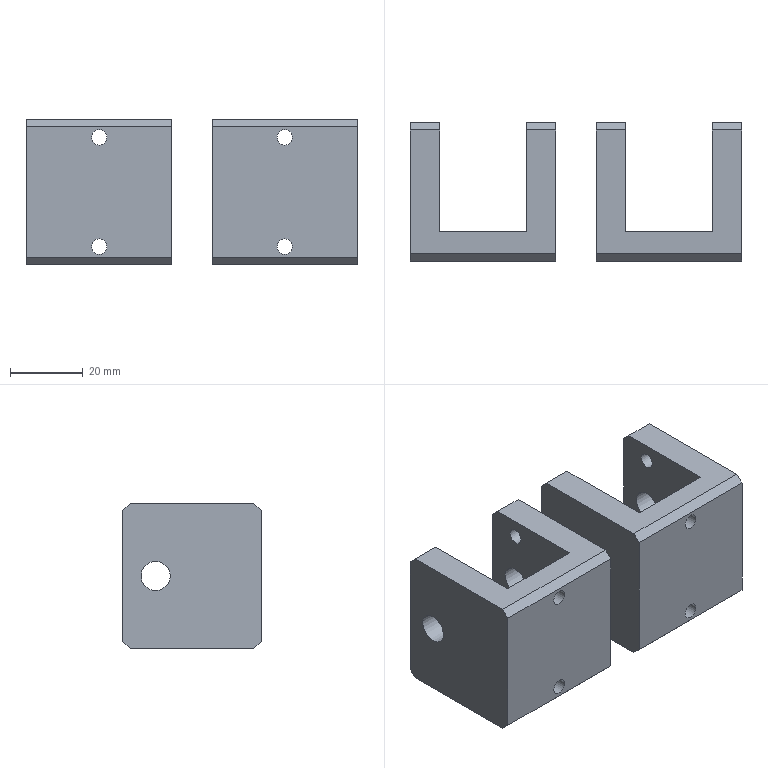NC program | NX | posted by the shop | part box 91 x 38 x 40 mm
Whole program:
%
O0001
(Machine time: 2.39 MIN)
(===Total Tool:3===)
(T1=D80R0.8 face mill D=80.  R=0.8  D-  H01 Z=0.    )
(T9=D10     D=10.  R=0.   D-  H09 Z=-2.   )
(T2=D6 chamfer mill   D=6.   R=0.   D-  H02 Z=-2.7  )
G80 G90 G17 G49 G40
G91 G28 Z0
M01
N1 T01 M06
(D80R0.8 face mill  D=80. R=0.8 H=01 ce=0.10 di=0.10)
G00 G90 G54 X97.597 Y-20. M03 S2800
G43 H01 Z20.
M08
Z3.525
G01 Z1.525 F3000.
X85.597
X-85.597
X-97.597
Z3.525
G00 X97.597
Z3.05
G01 Z1.05
X85.597
X-85.597
X-97.597
Z3.05
G00 X97.597
Z2.575
G01 Z.575
X85.597
X-85.597
X-97.597
Z2.575
G00 X97.597
Z2.1
G01 Z.1
X85.597
X-85.597
X-97.597
Z2.1
G00 Z20.
G91 G28 Z0.0
M05
M09
G91 G28 Z0.0
M01
N2 T01 M06
(D80R0.8 face mill-J  D=80. R=0.8 H=01 ce=0.00 di=0.00)
G00 G90 G54 X97.499 Y-20. M03 S4000
G43 H01 Z20.
M08
Z2.
G01 Z0.0 F1000.
X85.499
X-85.499
X-97.499
Z2.
G00 Z20.
G91 G28 Z0.0
M05
M09
G91 G28 Z0.0
M01
N3 T09 M06
(D10  D=10. R=0. H=09 ce=0.10 di=0.00)
G00 G90 G54 X0.0 Y7.219 M03 S7000
G43 H09 Z11.8
M08
Z.359
G01 Z-.141 F4000.
X-.57 Y3.093
X4.428 Y3.239
X4.513 Y3.241
X46.485
X46.572 Y3.239
Y3.312 Z-.212
Y3.38 Z-.283
X46.485 Y3.383
X4.513
X4.428 Y3.38
Y3.454 Z-.354
Y3.522 Z-.424
X4.513 Y3.524
X46.485
X46.572 Y3.522
X46.573 Y3.595 Z-.495
Y3.663 Z-.566
X46.485 Y3.666
X4.513
X4.428 Y3.663
X4.427 Y3.736 Z-.636
Y3.805 Z-.707
X4.513 Y3.807
X46.485
X46.573 Y3.805
Y3.878 Z-.778
Y3.946 Z-.849
X46.485 Y3.949
X4.513
X4.427 Y3.946
Y4.019 Z-.919
Y4.087 Z-.99
X4.513 Y4.09
X46.485
X46.573 Y4.087
Y4.161 Z-1.061
Y4.229 Z-1.131
X46.485 Y4.231
X4.513
X4.427 Y4.229
Y4.302 Z-1.202
Y4.37 Z-1.273
X4.513 Y4.373
X46.485
X46.573 Y4.37
Y4.444 Z-1.344
Y4.512 Z-1.414
X46.485 Y4.514
X4.513
X4.427 Y4.512
Y4.585 Z-1.485
X4.428 Y4.653 Z-1.556
X4.513 Y4.656
X46.485
X46.572 Y4.653
Y4.711 Z-1.611
Y4.764 Z-1.667
X46.485 Y4.767
X4.513
X4.428 Y4.764
Y4.822 Z-1.722
Y4.875 Z-1.778
X4.513 Y4.878
X46.485
X46.572 Y4.875
Y4.933 Z-1.833
Y4.986 Z-1.889
X46.485 Y4.989
X4.513
X4.428 Y4.986
Y5.044 Z-1.944
Y5.098 Z-2.
X46.572 Y5.097
G00 Z11.8
X-55.434 Y2.984
Z.359
G01 Z-.141
X-46.572 Y3.239
X-46.485 Y3.241
X-4.513
X-4.428 Y3.239
Y3.312 Z-.212
Y3.38 Z-.283
X-4.513 Y3.383
X-46.485
X-46.572 Y3.38
Y3.454 Z-.354
Y3.522 Z-.424
X-46.485 Y3.524
X-4.513
X-4.428 Y3.522
Y3.595 Z-.495
X-4.427 Y3.663 Z-.566
X-4.513 Y3.666
X-46.485
X-46.573 Y3.663
Y3.736 Z-.636
Y3.805 Z-.707
X-46.485 Y3.807
X-4.513
X-4.427 Y3.805
Y3.878 Z-.778
Y3.946 Z-.849
X-4.513 Y3.949
X-46.485
X-46.573 Y3.946
Y4.019 Z-.919
Y4.087 Z-.99
X-46.485 Y4.09
X-4.513
X-4.427 Y4.087
Y4.161 Z-1.061
Y4.229 Z-1.131
X-4.513 Y4.231
X-46.485
X-46.573 Y4.229
Y4.302 Z-1.202
Y4.37 Z-1.273
X-46.485 Y4.373
X-4.513
X-4.427 Y4.37
Y4.444 Z-1.344
Y4.512 Z-1.414
X-4.513 Y4.514
X-46.485
X-46.573 Y4.512
X-46.572 Y4.585 Z-1.485
Y4.653 Z-1.556
X-46.485 Y4.656
X-4.513
X-4.428 Y4.653
Y4.711 Z-1.611
Y4.764 Z-1.667
X-4.513 Y4.767
X-46.485
X-46.572 Y4.764
Y4.822 Z-1.722
Y4.875 Z-1.778
X-46.485 Y4.878
X-4.513
X-4.428 Y4.875
Y4.933 Z-1.833
Y4.986 Z-1.889
X-4.513 Y4.989
X-46.485
X-46.572 Y4.986
Y5.044 Z-1.944
Y5.097 Z-2.
X-4.428 Y5.098
G00 Z11.8
X55.434 Y-42.984
Z.359
G01 Z-.141
X46.572 Y-43.239
X46.485 Y-43.241
X4.513
X4.428 Y-43.239
Y-43.312 Z-.212
Y-43.38 Z-.283
X4.513 Y-43.383
X46.485
X46.572 Y-43.38
Y-43.454 Z-.354
Y-43.522 Z-.424
X46.485 Y-43.524
X4.513
X4.428 Y-43.522
Y-43.595 Z-.495
Y-43.663 Z-.566
X4.513 Y-43.666
X46.485
X46.573 Y-43.663
Y-43.736 Z-.636
Y-43.805 Z-.707
X46.485 Y-43.807
X4.513
X4.427 Y-43.805
Y-43.878 Z-.778
Y-43.946 Z-.849
X4.513 Y-43.949
X46.485
X46.573 Y-43.946
Y-44.019 Z-.919
Y-44.087 Z-.99
X46.485 Y-44.09
X4.513
X4.427 Y-44.087
Y-44.161 Z-1.061
Y-44.229 Z-1.131
X4.513 Y-44.231
X46.485
X46.573 Y-44.229
Y-44.302 Z-1.202
Y-44.37 Z-1.273
X46.485 Y-44.373
X4.513
X4.427 Y-44.37
Y-44.444 Z-1.344
Y-44.512 Z-1.414
X4.513 Y-44.514
X46.485
X46.573 Y-44.512
X46.572 Y-44.585 Z-1.485
Y-44.653 Z-1.556
X46.485 Y-44.656
X4.513
X4.428 Y-44.653
Y-44.711 Z-1.611
Y-44.764 Z-1.667
X4.513 Y-44.767
X46.485
X46.572 Y-44.764
Y-44.822 Z-1.722
Y-44.875 Z-1.778
X46.485 Y-44.878
X4.513
X4.428 Y-44.875
Y-44.933 Z-1.833
Y-44.986 Z-1.889
X4.513 Y-44.989
X46.485
X46.572 Y-44.986
Y-45.044 Z-1.944
Y-45.097 Z-2.
X46.485 Y-45.1
X4.513
X4.428 Y-45.098
G00 Z11.8
X0.0 Y-47.219
Z.359
G01 Z-.141
X.57 Y-43.093
X-4.428 Y-43.239
X-4.513 Y-43.241
X-46.485
X-46.572 Y-43.239
Y-43.312 Z-.212
Y-43.38 Z-.283
X-46.485 Y-43.383
X-4.513
X-4.428 Y-43.38
Y-43.454 Z-.354
Y-43.522 Z-.424
X-4.513 Y-43.524
X-46.485
X-46.572 Y-43.522
Y-43.595 Z-.495
X-46.573 Y-43.663 Z-.566
X-46.485 Y-43.666
X-4.513
X-4.427 Y-43.663
Y-43.736 Z-.636
Y-43.805 Z-.707
X-4.513 Y-43.807
X-46.485
X-46.573 Y-43.805
Y-43.878 Z-.778
Y-43.946 Z-.849
X-46.485 Y-43.949
X-4.513
X-4.427 Y-43.946
Y-44.019 Z-.919
Y-44.087 Z-.99
X-4.513 Y-44.09
X-46.485
X-46.573 Y-44.087
Y-44.161 Z-1.061
Y-44.229 Z-1.131
X-46.485 Y-44.231
X-4.513
X-4.427 Y-44.229
Y-44.302 Z-1.202
Y-44.37 Z-1.273
X-4.513 Y-44.373
X-46.485
X-46.573 Y-44.37
Y-44.444 Z-1.344
Y-44.512 Z-1.414
X-46.485 Y-44.514
X-4.513
X-4.427 Y-44.512
X-4.428 Y-44.585 Z-1.485
Y-44.653 Z-1.556
X-4.513 Y-44.656
X-46.485
X-46.572 Y-44.653
Y-44.711 Z-1.611
Y-44.764 Z-1.667
X-46.485 Y-44.767
X-4.513
X-4.428 Y-44.764
Y-44.822 Z-1.722
Y-44.875 Z-1.778
X-4.513 Y-44.878
X-46.485
X-46.572 Y-44.875
Y-44.933 Z-1.833
Y-44.986 Z-1.889
X-46.485 Y-44.989
X-4.513
X-4.428 Y-44.986
Y-45.044 Z-1.944
Y-45.098 Z-2.
X-4.513 Y-45.1
X-46.485
X-46.572 Y-45.097
G00 Z11.8
G91 G28 Z0.0
M05
M09
G91 G28 Z0.0
M01
N4 T02 M06
(D6 chamfer mill  D=6. R=0. H=02 ce=0.00 di=0.00)
G00 G90 G54 X-25.5 Y-35. M03 S8000
G43 H02 Z20.
M08
G98 G81 X-25.5 Y-35. Z-2.7 R3. F1000.
Y-5.
X25.5
Y-35.
G80
G00 Z20.
G00 G90 X-46.49 Y-38.792 M03 S6500
Z20.
Z.13
G01 Z-1.2 F1500.
G03 X-46.415 Y-38.452 I-1.907 J.601
G01 X-46.405 Y-38.398
X-46.428 Y-38.349
X-46.466 Y-38.259
X-46.5 Y-38.
Y-2.
X-46.466 Y-1.741
X-46.428 Y-1.651
X-46.405 Y-1.602
X-46.415 Y-1.548
G03 X-46.49 Y-1.208 I-1.983 J-.261
G01 Z.13
G00 Z10.
X-4.51
Z.13
G01 Z-1.2
G03 X-4.585 Y-1.548 I1.907 J-.601
G01 X-4.595 Y-1.602
X-4.572 Y-1.651
X-4.534 Y-1.741
X-4.5 Y-2.
Y-38.
X-4.534 Y-38.259
X-4.572 Y-38.349
X-4.595 Y-38.398
X-4.585 Y-38.452
G03 X-4.51 Y-38.792 I1.983 J.261
G01 Z.13
G00 Z10.
X46.49 Y-1.208
Z.13
G01 Z-1.2
G03 X46.415 Y-1.548 I1.907 J-.601
G01 X46.405 Y-1.602
X46.428 Y-1.651
X46.466 Y-1.741
X46.5 Y-2.
Y-38.
X46.466 Y-38.259
X46.428 Y-38.349
X46.405 Y-38.398
X46.415 Y-38.452
G03 X46.49 Y-38.792 I1.983 J.261
G01 Z.13
G00 Z10.
X4.51
Z.13
G01 Z-1.2
G03 X4.585 Y-38.452 I-1.907 J.601
G01 X4.595 Y-38.398
X4.572 Y-38.349
X4.534 Y-38.259
X4.5 Y-38.
Y-20.
Y-2.
X4.534 Y-1.741
X4.572 Y-1.651
X4.595 Y-1.602
X4.585 Y-1.548
G03 X4.51 Y-1.208 I-1.983 J-.261
G01 Z.13
G00 Z20.
G00 G90 X-1.6 Y-41.516 M03 S6500
Z20.
Z-1.2
G01 Z-2.7 F1000.
G03 X-2.737 Y-40.7 I-1.137 J-.384
G01 X-48.263
G03 X-49.4 Y-41.516 I0.0 J-1.2
G01 Z-1.2
G00 Z20.
X49.4
Z-1.2
G01 Z-2.7
G03 X48.263 Y-40.7 I-1.137 J-.384
G01 X2.737
G03 X1.6 Y-41.516 I0.0 J-1.2
G01 Z-1.2
G00 Z20.
X-49.4 Y1.516
Z-1.2
G01 Z-2.7
G03 X-48.263 Y.7 I1.137 J.384
G01 X-2.737
G03 X-1.6 Y1.516 I0.0 J1.2
G01 Z-1.2
G00 Z20.
X1.6
Z-1.2
G01 Z-2.7
G03 X2.737 Y.7 I1.137 J.384
G01 X48.263
G03 X49.4 Y1.516 I0.0 J1.2
G01 Z-1.2
G00 Z20.
M05
M09
G91 G28 Z0.0
G91 G28 Y0.0
M30
%